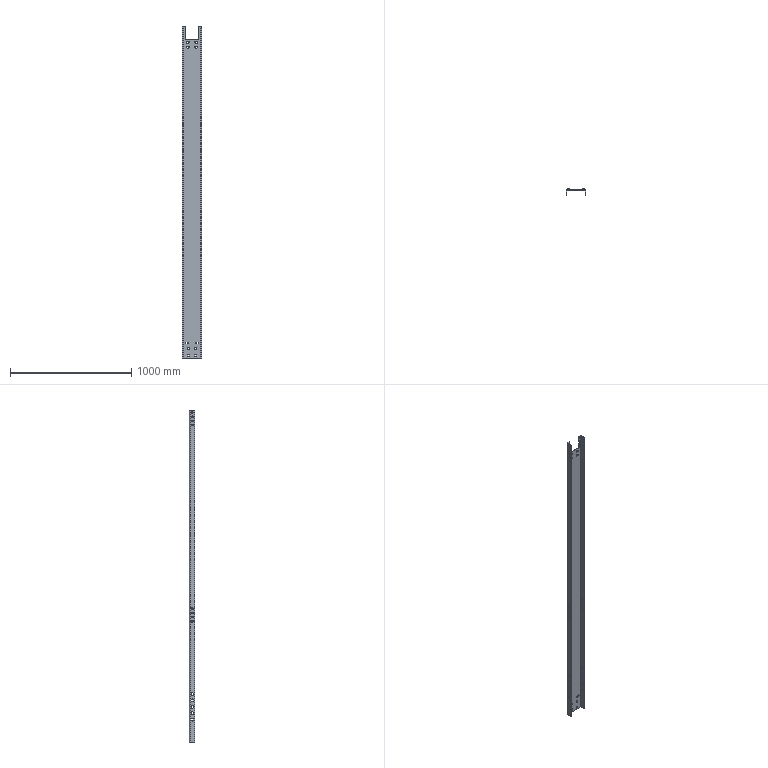Part | SolidWorks | features ICE 3, Cut 1, Fillet 1, FlatPattern 1, SMBaseFlange 1, SheetMetal 1 | 1 solid | 144 faces | box 160 x 45 x 2739 mm | volume 3145036 mm3 | cylinder 82 | plane 62 | commonest cylinder face diameters 14 x42 13 x28 11 x8 2 x2 12 x2